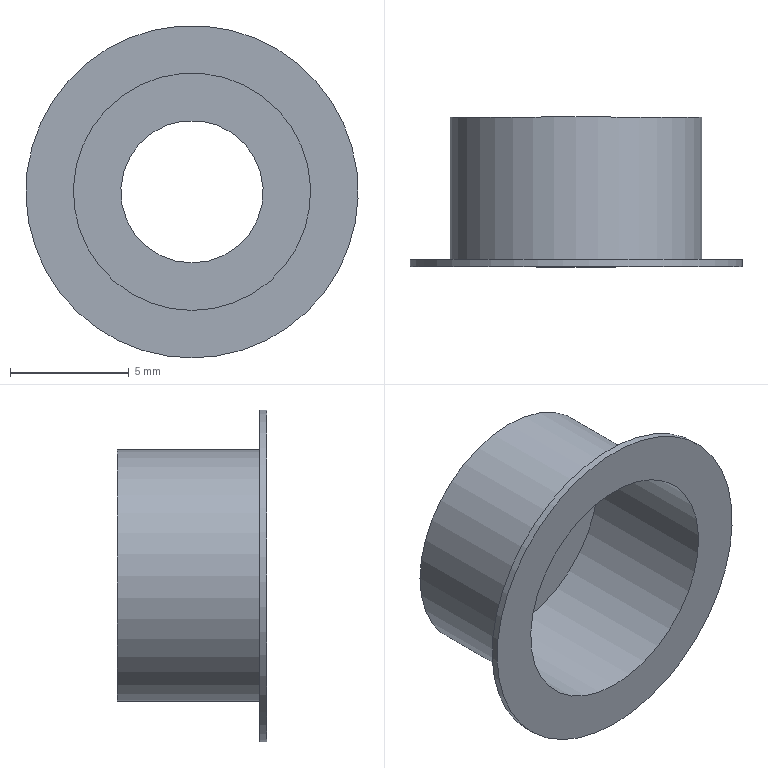Part | NX | features DATUM_CSYS 2, SKETCH 1, SWP104 1 | 1 solid | 8 faces | box 14 x 6.3 x 14 mm | volume 95.944 mm3 | cylinder 4 | plane 4 | commonest cylinder face diameters 6 x1 10 x1 10.6 x1 14 x1
STEP:
#1=CARTESIAN_POINT('',(0.,0.3,-5.3));
#2=VERTEX_POINT('',#1);
#3=CARTESIAN_POINT('',(0.,0.3,0.));
#4=DIRECTION('',(0.,-1.,0.));
#5=DIRECTION('',(0.,0.,-1.));
#6=AXIS2_PLACEMENT_3D('',#3,#4,#5);
#7=CIRCLE('',#6,5.3);
#8=EDGE_CURVE('',#2,#2,#7,.T.);
#9=ORIENTED_EDGE('',*,*,#8,.F.);
#10=EDGE_LOOP('',(#9));
#11=FACE_BOUND('',#10,.T.);
#12=CARTESIAN_POINT('',(0.,6.3,-5.3));
#13=VERTEX_POINT('',#12);
#14=CARTESIAN_POINT('',(0.,6.3,0.));
#15=DIRECTION('',(0.,-1.,0.));
#16=DIRECTION('',(0.,0.,-1.));
#17=AXIS2_PLACEMENT_3D('',#14,#15,#16);
#18=CIRCLE('',#17,5.3);
#19=EDGE_CURVE('',#13,#13,#18,.T.);
#20=ORIENTED_EDGE('',*,*,#19,.T.);
#21=EDGE_LOOP('',(#20));
#22=FACE_BOUND('',#21,.T.);
#23=CARTESIAN_POINT('',(0.,0.,0.));
#24=DIRECTION('',(0.,-1.,0.));
#25=DIRECTION('',(0.,0.,-1.));
#26=AXIS2_PLACEMENT_3D('',#23,#24,#25);
#27=CYLINDRICAL_SURFACE('',#26,5.3);
#28=ADVANCED_FACE('',(#11,#22),#27,.T.);
#29=CARTESIAN_POINT('',(0.,0.3,-7.));
#30=VERTEX_POINT('',#29);
#31=CARTESIAN_POINT('',(0.,0.3,0.));
#32=DIRECTION('',(0.,-1.,0.));
#33=DIRECTION('',(0.,0.,-1.));
#34=AXIS2_PLACEMENT_3D('',#31,#32,#33);
#35=CIRCLE('',#34,7.);
#36=EDGE_CURVE('',#30,#30,#35,.T.);
#37=ORIENTED_EDGE('',*,*,#36,.F.);
#38=EDGE_LOOP('',(#37));
#39=FACE_BOUND('',#38,.T.);
#40=ORIENTED_EDGE('',*,*,#8,.T.);
#41=EDGE_LOOP('',(#40));
#42=FACE_BOUND('',#41,.T.);
#43=CARTESIAN_POINT('',(0.,0.3,5.3));
#44=DIRECTION('',(0.,-1.,0.));
#45=DIRECTION('',(0.,0.,-1.));
#46=AXIS2_PLACEMENT_3D('',#43,#44,#45);
#47=PLANE('',#46);
#48=ADVANCED_FACE('',(#39,#42),#47,.F.);
#49=CARTESIAN_POINT('',(0.,0.,-7.));
#50=VERTEX_POINT('',#49);
#51=CARTESIAN_POINT('',(0.,0.,0.));
#52=DIRECTION('',(0.,-1.,0.));
#53=DIRECTION('',(0.,0.,-1.));
#54=AXIS2_PLACEMENT_3D('',#51,#52,#53);
#55=CIRCLE('',#54,7.);
#56=EDGE_CURVE('',#50,#50,#55,.T.);
#57=ORIENTED_EDGE('',*,*,#56,.F.);
#58=EDGE_LOOP('',(#57));
#59=FACE_BOUND('',#58,.T.);
#60=ORIENTED_EDGE('',*,*,#36,.T.);
#61=EDGE_LOOP('',(#60));
#62=FACE_BOUND('',#61,.T.);
#63=CARTESIAN_POINT('',(0.,0.,0.));
#64=DIRECTION('',(0.,-1.,0.));
#65=DIRECTION('',(0.,0.,-1.));
#66=AXIS2_PLACEMENT_3D('',#63,#64,#65);
#67=CYLINDRICAL_SURFACE('',#66,7.);
#68=ADVANCED_FACE('',(#59,#62),#67,.T.);
#69=CARTESIAN_POINT('',(0.,0.,-5.));
#70=VERTEX_POINT('',#69);
#71=CARTESIAN_POINT('',(0.,0.,0.));
#72=DIRECTION('',(0.,-1.,0.));
#73=DIRECTION('',(0.,0.,-1.));
#74=AXIS2_PLACEMENT_3D('',#71,#72,#73);
#75=CIRCLE('',#74,5.);
#76=EDGE_CURVE('',#70,#70,#75,.T.);
#77=ORIENTED_EDGE('',*,*,#76,.F.);
#78=EDGE_LOOP('',(#77));
#79=FACE_BOUND('',#78,.T.);
#80=ORIENTED_EDGE('',*,*,#56,.T.);
#81=EDGE_LOOP('',(#80));
#82=FACE_BOUND('',#81,.T.);
#83=CARTESIAN_POINT('',(0.,0.,7.));
#84=DIRECTION('',(0.,1.,0.));
#85=DIRECTION('',(0.,0.,1.));
#86=AXIS2_PLACEMENT_3D('',#83,#84,#85);
#87=PLANE('',#86);
#88=ADVANCED_FACE('',(#79,#82),#87,.F.);
#89=CARTESIAN_POINT('',(0.,6.,-5.));
#90=VERTEX_POINT('',#89);
#91=CARTESIAN_POINT('',(0.,6.,0.));
#92=DIRECTION('',(0.,-1.,0.));
#93=DIRECTION('',(0.,0.,-1.));
#94=AXIS2_PLACEMENT_3D('',#91,#92,#93);
#95=CIRCLE('',#94,5.);
#96=EDGE_CURVE('',#90,#90,#95,.T.);
#97=ORIENTED_EDGE('',*,*,#96,.F.);
#98=EDGE_LOOP('',(#97));
#99=FACE_BOUND('',#98,.T.);
#100=ORIENTED_EDGE('',*,*,#76,.T.);
#101=EDGE_LOOP('',(#100));
#102=FACE_BOUND('',#101,.T.);
#103=CARTESIAN_POINT('',(0.,0.,0.));
#104=DIRECTION('',(0.,-1.,0.));
#105=DIRECTION('',(0.,0.,-1.));
#106=AXIS2_PLACEMENT_3D('',#103,#104,#105);
#107=CYLINDRICAL_SURFACE('',#106,5.);
#108=ADVANCED_FACE('',(#99,#102),#107,.F.);
#109=CARTESIAN_POINT('',(0.,6.,-3.));
#110=VERTEX_POINT('',#109);
#111=CARTESIAN_POINT('',(0.,6.,0.));
#112=DIRECTION('',(0.,-1.,0.));
#113=DIRECTION('',(0.,0.,-1.));
#114=AXIS2_PLACEMENT_3D('',#111,#112,#113);
#115=CIRCLE('',#114,3.);
#116=EDGE_CURVE('',#110,#110,#115,.T.);
#117=ORIENTED_EDGE('',*,*,#116,.F.);
#118=EDGE_LOOP('',(#117));
#119=FACE_BOUND('',#118,.T.);
#120=ORIENTED_EDGE('',*,*,#96,.T.);
#121=EDGE_LOOP('',(#120));
#122=FACE_BOUND('',#121,.T.);
#123=CARTESIAN_POINT('',(0.,6.,5.));
#124=DIRECTION('',(0.,1.,0.));
#125=DIRECTION('',(0.,0.,1.));
#126=AXIS2_PLACEMENT_3D('',#123,#124,#125);
#127=PLANE('',#126);
#128=ADVANCED_FACE('',(#119,#122),#127,.F.);
#129=CARTESIAN_POINT('',(0.,6.3,-3.));
#130=VERTEX_POINT('',#129);
#131=CARTESIAN_POINT('',(0.,6.3,0.));
#132=DIRECTION('',(0.,-1.,0.));
#133=DIRECTION('',(0.,0.,-1.));
#134=AXIS2_PLACEMENT_3D('',#131,#132,#133);
#135=CIRCLE('',#134,3.);
#136=EDGE_CURVE('',#130,#130,#135,.T.);
#137=ORIENTED_EDGE('',*,*,#136,.F.);
#138=EDGE_LOOP('',(#137));
#139=FACE_BOUND('',#138,.T.);
#140=ORIENTED_EDGE('',*,*,#116,.T.);
#141=EDGE_LOOP('',(#140));
#142=FACE_BOUND('',#141,.T.);
#143=CARTESIAN_POINT('',(0.,0.,0.));
#144=DIRECTION('',(0.,-1.,0.));
#145=DIRECTION('',(0.,0.,-1.));
#146=AXIS2_PLACEMENT_3D('',#143,#144,#145);
#147=CYLINDRICAL_SURFACE('',#146,3.);
#148=ADVANCED_FACE('',(#139,#142),#147,.F.);
#149=ORIENTED_EDGE('',*,*,#19,.F.);
#150=EDGE_LOOP('',(#149));
#151=FACE_BOUND('',#150,.T.);
#152=ORIENTED_EDGE('',*,*,#136,.T.);
#153=EDGE_LOOP('',(#152));
#154=FACE_BOUND('',#153,.T.);
#155=CARTESIAN_POINT('',(0.,6.3,3.));
#156=DIRECTION('',(0.,-1.,0.));
#157=DIRECTION('',(0.,0.,-1.));
#158=AXIS2_PLACEMENT_3D('',#155,#156,#157);
#159=PLANE('',#158);
#160=ADVANCED_FACE('',(#151,#154),#159,.F.);
#161=CLOSED_SHELL('',(#28,#48,#68,#88,#108,#128,#148,#160));
#162=MANIFOLD_SOLID_BREP('',#161);
#163=(LENGTH_UNIT()NAMED_UNIT(*)SI_UNIT(.MILLI.,.METRE.));
#164=UNCERTAINTY_MEASURE_WITH_UNIT(LENGTH_MEASURE(0.00001),#163,'','');
#165=(NAMED_UNIT(*)PLANE_ANGLE_UNIT()SI_UNIT($,.RADIAN.));
#166=(NAMED_UNIT(*)SI_UNIT($,.STERADIAN.)SOLID_ANGLE_UNIT());
#167=(GEOMETRIC_REPRESENTATION_CONTEXT(3)GLOBAL_UNCERTAINTY_ASSIGNED_CONTEXT((#164))GLOBAL_UNIT_ASSIGNED_CONTEXT((#163,#165,#166))REPRESENTATION_CONTEXT('',''));
#168=ADVANCED_BREP_SHAPE_REPRESENTATION('',(#162),#167);